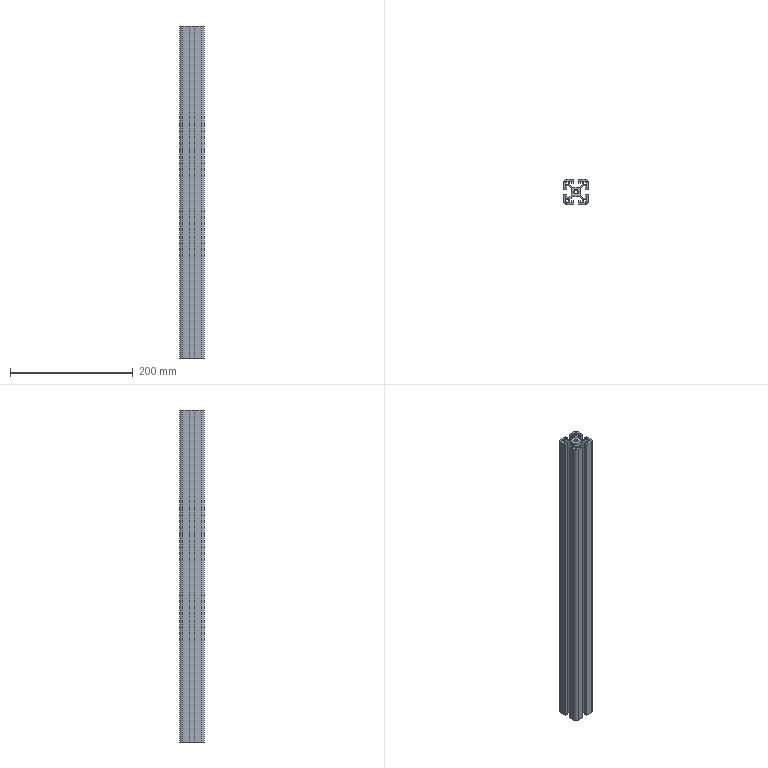Part | STEP file | 4040-540 | 1 solid | 88 faces | box 40 x 40 x 540 mm | volume 380131 mm3 | plane 78 | cylinder 10 | commonest cylinder face diameters 4 x4 10 x4 6.8 x2